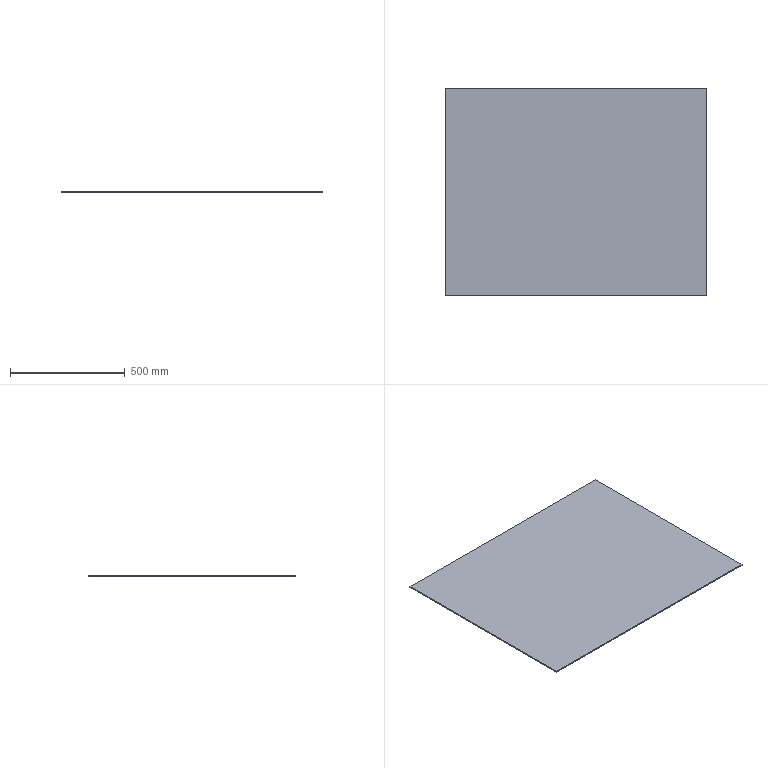Part | SolidWorks | features Extrusion 1, HoleWzd 1 | 1 solid | 6 faces | box 1142 x 906 x 5 mm | volume 5173260 mm3 | plane 6
STEP:
#1=CARTESIAN_POINT('',(571.,-453.,0.));
#2=VERTEX_POINT('',#1);
#3=CARTESIAN_POINT('',(571.,453.,0.));
#4=VERTEX_POINT('',#3);
#5=CARTESIAN_POINT('',(571.,453.,0.));
#6=DIRECTION('',(0.,1.,0.));
#7=VECTOR('',#6,1000.);
#8=LINE('',#5,#7);
#9=EDGE_CURVE('',#2,#4,#8,.T.);
#10=ORIENTED_EDGE('',*,*,#9,.T.);
#11=CARTESIAN_POINT('',(571.,453.,5.));
#12=VERTEX_POINT('',#11);
#13=CARTESIAN_POINT('',(571.,453.,5.));
#14=DIRECTION('',(0.,0.,-1.));
#15=VECTOR('',#14,1000.);
#16=LINE('',#13,#15);
#17=EDGE_CURVE('',#12,#4,#16,.T.);
#18=ORIENTED_EDGE('',*,*,#17,.F.);
#19=CARTESIAN_POINT('',(571.,-453.,5.));
#20=VERTEX_POINT('',#19);
#21=CARTESIAN_POINT('',(571.,453.,5.));
#22=DIRECTION('',(0.,1.,0.));
#23=VECTOR('',#22,1000.);
#24=LINE('',#21,#23);
#25=EDGE_CURVE('',#20,#12,#24,.T.);
#26=ORIENTED_EDGE('',*,*,#25,.F.);
#27=CARTESIAN_POINT('',(571.,-453.,5.));
#28=DIRECTION('',(0.,0.,-1.));
#29=VECTOR('',#28,1000.);
#30=LINE('',#27,#29);
#31=EDGE_CURVE('',#20,#2,#30,.T.);
#32=ORIENTED_EDGE('',*,*,#31,.T.);
#33=EDGE_LOOP('',(#10,#18,#26,#32));
#34=FACE_OUTER_BOUND('',#33,.T.);
#35=CARTESIAN_POINT('',(571.,453.,5.));
#36=DIRECTION('',(-1.,0.,0.));
#37=DIRECTION('',(0.,-1.,0.));
#38=AXIS2_PLACEMENT_3D('',#35,#36,#37);
#39=PLANE('',#38);
#40=ADVANCED_FACE('',(#34),#39,.F.);
#41=CARTESIAN_POINT('',(-571.,453.,0.));
#42=VERTEX_POINT('',#41);
#43=CARTESIAN_POINT('',(-571.,453.,0.));
#44=DIRECTION('',(-1.,0.,0.));
#45=VECTOR('',#44,1000.);
#46=LINE('',#43,#45);
#47=EDGE_CURVE('',#4,#42,#46,.T.);
#48=ORIENTED_EDGE('',*,*,#47,.T.);
#49=CARTESIAN_POINT('',(-571.,453.,5.));
#50=VERTEX_POINT('',#49);
#51=CARTESIAN_POINT('',(-571.,453.,5.));
#52=DIRECTION('',(0.,0.,-1.));
#53=VECTOR('',#52,1000.);
#54=LINE('',#51,#53);
#55=EDGE_CURVE('',#50,#42,#54,.T.);
#56=ORIENTED_EDGE('',*,*,#55,.F.);
#57=CARTESIAN_POINT('',(-571.,453.,5.));
#58=DIRECTION('',(-1.,0.,0.));
#59=VECTOR('',#58,1000.);
#60=LINE('',#57,#59);
#61=EDGE_CURVE('',#12,#50,#60,.T.);
#62=ORIENTED_EDGE('',*,*,#61,.F.);
#63=ORIENTED_EDGE('',*,*,#17,.T.);
#64=EDGE_LOOP('',(#48,#56,#62,#63));
#65=FACE_OUTER_BOUND('',#64,.T.);
#66=CARTESIAN_POINT('',(-571.,453.,5.));
#67=DIRECTION('',(0.,-1.,0.));
#68=DIRECTION('',(0.,0.,-1.));
#69=AXIS2_PLACEMENT_3D('',#66,#67,#68);
#70=PLANE('',#69);
#71=ADVANCED_FACE('',(#65),#70,.F.);
#72=CARTESIAN_POINT('',(-571.,-453.,0.));
#73=VERTEX_POINT('',#72);
#74=CARTESIAN_POINT('',(-571.,453.,0.));
#75=DIRECTION('',(0.,-1.,0.));
#76=VECTOR('',#75,1000.);
#77=LINE('',#74,#76);
#78=EDGE_CURVE('',#42,#73,#77,.T.);
#79=ORIENTED_EDGE('',*,*,#78,.T.);
#80=CARTESIAN_POINT('',(-571.,-453.,5.));
#81=VERTEX_POINT('',#80);
#82=CARTESIAN_POINT('',(-571.,-453.,5.));
#83=DIRECTION('',(0.,0.,-1.));
#84=VECTOR('',#83,1000.);
#85=LINE('',#82,#84);
#86=EDGE_CURVE('',#81,#73,#85,.T.);
#87=ORIENTED_EDGE('',*,*,#86,.F.);
#88=CARTESIAN_POINT('',(-571.,453.,5.));
#89=DIRECTION('',(0.,-1.,0.));
#90=VECTOR('',#89,1000.);
#91=LINE('',#88,#90);
#92=EDGE_CURVE('',#50,#81,#91,.T.);
#93=ORIENTED_EDGE('',*,*,#92,.F.);
#94=ORIENTED_EDGE('',*,*,#55,.T.);
#95=EDGE_LOOP('',(#79,#87,#93,#94));
#96=FACE_OUTER_BOUND('',#95,.T.);
#97=CARTESIAN_POINT('',(-571.,453.,5.));
#98=DIRECTION('',(1.,0.,0.));
#99=DIRECTION('',(0.,1.,0.));
#100=AXIS2_PLACEMENT_3D('',#97,#98,#99);
#101=PLANE('',#100);
#102=ADVANCED_FACE('',(#96),#101,.F.);
#103=CARTESIAN_POINT('',(-571.,-453.,0.));
#104=DIRECTION('',(1.,0.,0.));
#105=VECTOR('',#104,1000.);
#106=LINE('',#103,#105);
#107=EDGE_CURVE('',#73,#2,#106,.T.);
#108=ORIENTED_EDGE('',*,*,#107,.T.);
#109=ORIENTED_EDGE('',*,*,#31,.F.);
#110=CARTESIAN_POINT('',(-571.,-453.,5.));
#111=DIRECTION('',(1.,0.,0.));
#112=VECTOR('',#111,1000.);
#113=LINE('',#110,#112);
#114=EDGE_CURVE('',#81,#20,#113,.T.);
#115=ORIENTED_EDGE('',*,*,#114,.F.);
#116=ORIENTED_EDGE('',*,*,#86,.T.);
#117=EDGE_LOOP('',(#108,#109,#115,#116));
#118=FACE_OUTER_BOUND('',#117,.T.);
#119=CARTESIAN_POINT('',(-571.,-453.,5.));
#120=DIRECTION('',(0.,1.,0.));
#121=DIRECTION('',(0.,0.,1.));
#122=AXIS2_PLACEMENT_3D('',#119,#120,#121);
#123=PLANE('',#122);
#124=ADVANCED_FACE('',(#118),#123,.F.);
#125=ORIENTED_EDGE('',*,*,#25,.T.);
#126=ORIENTED_EDGE('',*,*,#61,.T.);
#127=ORIENTED_EDGE('',*,*,#92,.T.);
#128=ORIENTED_EDGE('',*,*,#114,.T.);
#129=EDGE_LOOP('',(#125,#126,#127,#128));
#130=FACE_OUTER_BOUND('',#129,.T.);
#131=CARTESIAN_POINT('',(0.,0.,5.));
#132=DIRECTION('',(0.,0.,1.));
#133=DIRECTION('',(1.,0.,0.));
#134=AXIS2_PLACEMENT_3D('',#131,#132,#133);
#135=PLANE('',#134);
#136=ADVANCED_FACE('',(#130),#135,.T.);
#137=ORIENTED_EDGE('',*,*,#9,.F.);
#138=ORIENTED_EDGE('',*,*,#107,.F.);
#139=ORIENTED_EDGE('',*,*,#78,.F.);
#140=ORIENTED_EDGE('',*,*,#47,.F.);
#141=EDGE_LOOP('',(#137,#138,#139,#140));
#142=FACE_OUTER_BOUND('',#141,.T.);
#143=CARTESIAN_POINT('',(0.,0.,0.));
#144=DIRECTION('',(0.,0.,1.));
#145=DIRECTION('',(1.,0.,0.));
#146=AXIS2_PLACEMENT_3D('',#143,#144,#145);
#147=PLANE('',#146);
#148=ADVANCED_FACE('',(#142),#147,.F.);
#149=CLOSED_SHELL('',(#40,#71,#102,#124,#136,#148));
#150=MANIFOLD_SOLID_BREP('',#149);
#151=CARTESIAN_POINT('',(0.,0.,0.));
#152=DIRECTION('',(0.,0.,1.));
#153=DIRECTION('',(1.,0.,0.));
#154=AXIS2_PLACEMENT_3D('',#151,#152,#153);
#155=(LENGTH_UNIT()NAMED_UNIT(*)SI_UNIT(.MILLI.,.METRE.));
#156=UNCERTAINTY_MEASURE_WITH_UNIT(LENGTH_MEASURE(0.00001),#155,'','');
#157=(NAMED_UNIT(*)PLANE_ANGLE_UNIT()SI_UNIT($,.RADIAN.));
#158=(NAMED_UNIT(*)SI_UNIT($,.STERADIAN.)SOLID_ANGLE_UNIT());
#159=(GEOMETRIC_REPRESENTATION_CONTEXT(3)GLOBAL_UNCERTAINTY_ASSIGNED_CONTEXT((#156))GLOBAL_UNIT_ASSIGNED_CONTEXT((#155,#157,#158))REPRESENTATION_CONTEXT('',''));
#160=ADVANCED_BREP_SHAPE_REPRESENTATION('',(#150,#154),#159);